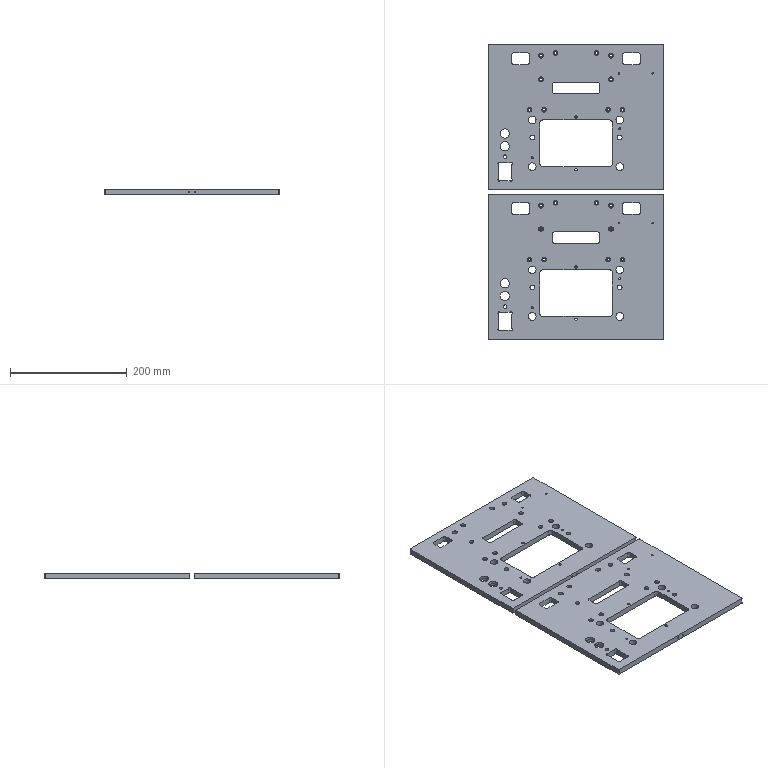Part | 2 solids | 792 faces | box 300 x 507 x 10 mm | volume 1195200 mm3 | plane 404 | cylinder 236 | spline 128 | cone 24 | commonest cylinder face diameters 8 x48 4.5 x40 2.5 x32 6 x28 13 x16 2 x12